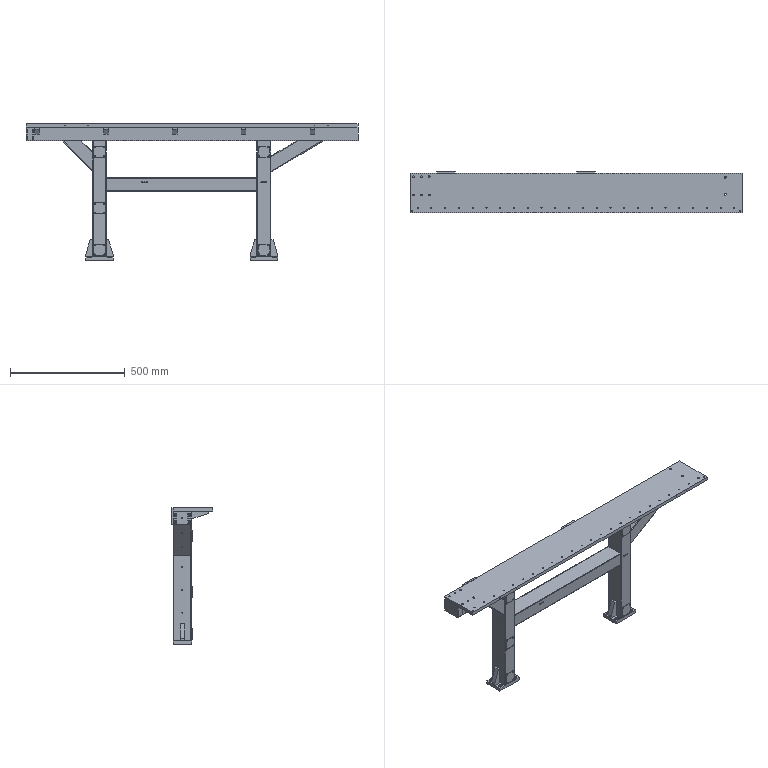Part | NX | 25 solids | 434 faces | box 1446 x 180 x 595 mm | volume 9755424 mm3 | plane 237 | cylinder 179 | cone 18 | commonest cylinder face diameters 5 x58 5.236 x48 4.2 x23 3.3 x20 9 x8 18 x8